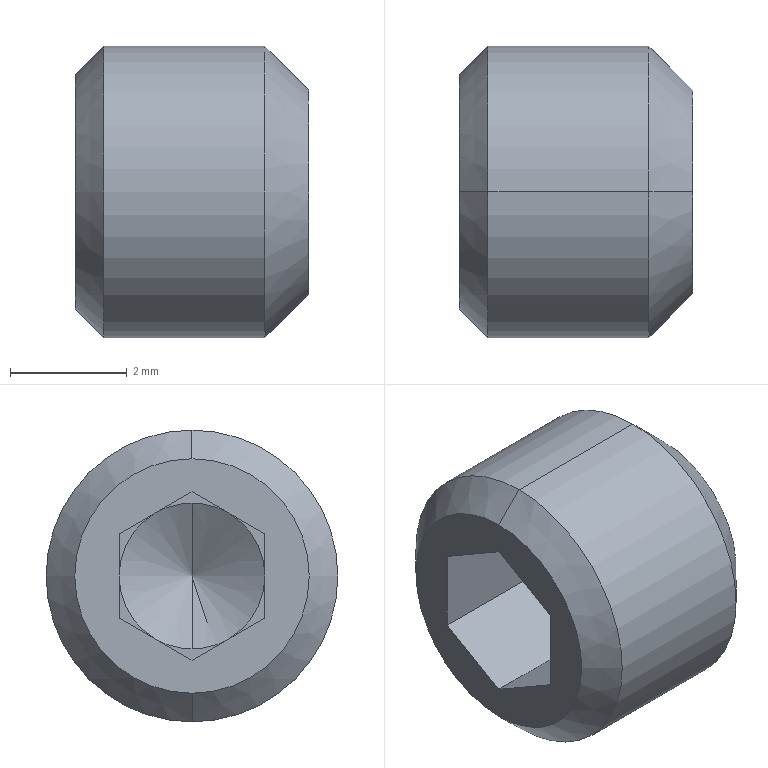Part | SolidWorks | features BaseBody 1 | 1 solid | 22 faces | box 4 x 5 x 5 mm | volume 60.792 mm3 | plane 14 | cone 6 | cylinder 2 | commonest cylinder face diameters 5 x2